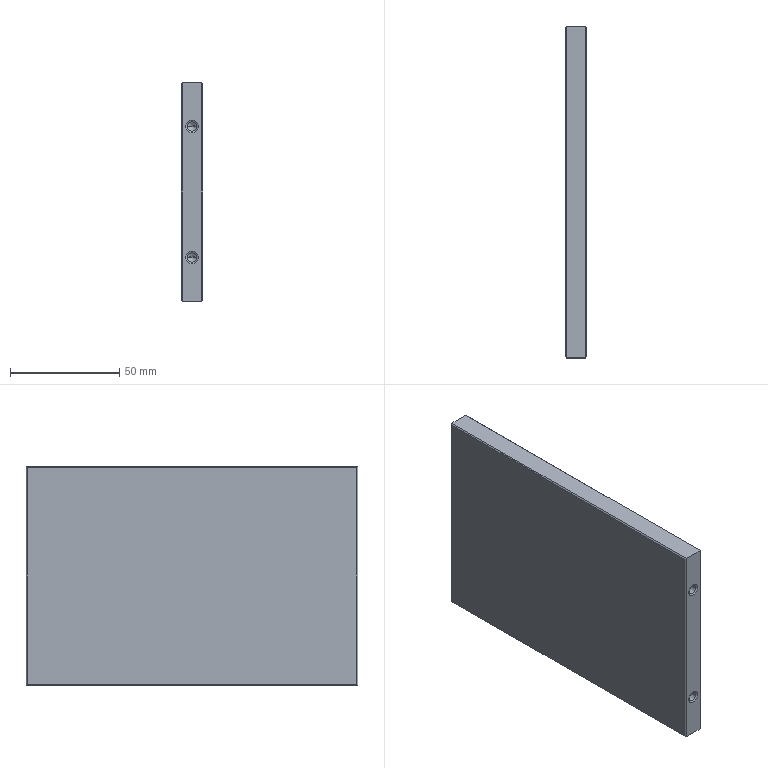Part | NX | 1 solid | 38 faces | box 10 x 151.9 x 100 mm | volume 150921 mm3 | cone 16 | plane 14 | cylinder 8 | commonest cylinder face diameters 4.2 x8
STEP:
#1=CARTESIAN_POINT('',(-4.5,-74.75,0.));
#2=VERTEX_POINT('',#1);
#3=CARTESIAN_POINT('',(4.5,-74.75,0.));
#4=VERTEX_POINT('',#3);
#5=CARTESIAN_POINT('',(0.,-74.75,0.));
#6=DIRECTION('',(1.,0.,0.));
#7=VECTOR('',#6,1000.);
#8=LINE('',#5,#7);
#9=EDGE_CURVE('',#2,#4,#8,.T.);
#10=ORIENTED_EDGE('',*,*,#9,.F.);
#11=CARTESIAN_POINT('',(-4.5,77.15,0.));
#12=VERTEX_POINT('',#11);
#13=CARTESIAN_POINT('',(-4.5,0.,0.));
#14=DIRECTION('',(0.,-1.,0.));
#15=VECTOR('',#14,1000.);
#16=LINE('',#13,#15);
#17=EDGE_CURVE('',#12,#2,#16,.T.);
#18=ORIENTED_EDGE('',*,*,#17,.F.);
#19=CARTESIAN_POINT('',(4.5,77.15,0.));
#20=VERTEX_POINT('',#19);
#21=CARTESIAN_POINT('',(0.,77.15,0.));
#22=DIRECTION('',(-1.,0.,0.));
#23=VECTOR('',#22,1000.);
#24=LINE('',#21,#23);
#25=EDGE_CURVE('',#20,#12,#24,.T.);
#26=ORIENTED_EDGE('',*,*,#25,.F.);
#27=CARTESIAN_POINT('',(4.5,0.,0.));
#28=DIRECTION('',(0.,1.,0.));
#29=VECTOR('',#28,1000.);
#30=LINE('',#27,#29);
#31=EDGE_CURVE('',#4,#20,#30,.T.);
#32=ORIENTED_EDGE('',*,*,#31,.F.);
#33=EDGE_LOOP('',(#10,#18,#26,#32));
#34=FACE_BOUND('',#33,.T.);
#35=CARTESIAN_POINT('',(0.,0.,0.));
#36=DIRECTION('',(0.,0.,1.));
#37=DIRECTION('',(1.,0.,0.));
#38=AXIS2_PLACEMENT_3D('',#35,#36,#37);
#39=PLANE('',#38);
#40=ADVANCED_FACE('',(#34),#39,.F.);
#41=CARTESIAN_POINT('',(-5.,-74.25,0.5));
#42=VERTEX_POINT('',#41);
#43=CARTESIAN_POINT('',(-4.5,-74.75,0.));
#44=DIRECTION('',(0.5774,-0.5774,-0.5774));
#45=VECTOR('',#44,1000.);
#46=LINE('',#43,#45);
#47=EDGE_CURVE('',#42,#2,#46,.T.);
#48=ORIENTED_EDGE('',*,*,#47,.F.);
#49=CARTESIAN_POINT('',(-5.,76.65,0.5));
#50=VERTEX_POINT('',#49);
#51=CARTESIAN_POINT('',(-5.,0.,0.5));
#52=DIRECTION('',(0.,-1.,0.));
#53=VECTOR('',#52,1000.);
#54=LINE('',#51,#53);
#55=EDGE_CURVE('',#50,#42,#54,.T.);
#56=ORIENTED_EDGE('',*,*,#55,.F.);
#57=CARTESIAN_POINT('',(-4.5,77.15,0.));
#58=DIRECTION('',(-0.5774,-0.5774,0.5774));
#59=VECTOR('',#58,1000.);
#60=LINE('',#57,#59);
#61=EDGE_CURVE('',#12,#50,#60,.T.);
#62=ORIENTED_EDGE('',*,*,#61,.F.);
#63=ORIENTED_EDGE('',*,*,#17,.T.);
#64=EDGE_LOOP('',(#48,#56,#62,#63));
#65=FACE_BOUND('',#64,.T.);
#66=CARTESIAN_POINT('',(-4.5,76.65,0.));
#67=DIRECTION('',(-0.7071,0.,-0.7071));
#68=DIRECTION('',(-0.7071,0.,0.7071));
#69=AXIS2_PLACEMENT_3D('',#66,#67,#68);
#70=PLANE('',#69);
#71=ADVANCED_FACE('',(#65),#70,.T.);
#72=CARTESIAN_POINT('',(5.,76.65,0.5));
#73=VERTEX_POINT('',#72);
#74=CARTESIAN_POINT('',(5.,-74.25,0.5));
#75=VERTEX_POINT('',#74);
#76=CARTESIAN_POINT('',(5.,0.,0.5));
#77=DIRECTION('',(0.,-1.,0.));
#78=VECTOR('',#77,1000.);
#79=LINE('',#76,#78);
#80=EDGE_CURVE('',#73,#75,#79,.T.);
#81=ORIENTED_EDGE('',*,*,#80,.F.);
#82=CARTESIAN_POINT('',(5.,76.65,99.5));
#83=VERTEX_POINT('',#82);
#84=CARTESIAN_POINT('',(5.,76.65,0.));
#85=DIRECTION('',(0.,0.,-1.));
#86=VECTOR('',#85,1000.);
#87=LINE('',#84,#86);
#88=EDGE_CURVE('',#83,#73,#87,.T.);
#89=ORIENTED_EDGE('',*,*,#88,.F.);
#90=CARTESIAN_POINT('',(5.,-74.25,99.5));
#91=VERTEX_POINT('',#90);
#92=CARTESIAN_POINT('',(5.,0.,99.5));
#93=DIRECTION('',(0.,-1.,0.));
#94=VECTOR('',#93,1000.);
#95=LINE('',#92,#94);
#96=EDGE_CURVE('',#83,#91,#95,.T.);
#97=ORIENTED_EDGE('',*,*,#96,.T.);
#98=CARTESIAN_POINT('',(5.,-74.25,0.));
#99=DIRECTION('',(0.,0.,1.));
#100=VECTOR('',#99,1000.);
#101=LINE('',#98,#100);
#102=EDGE_CURVE('',#75,#91,#101,.T.);
#103=ORIENTED_EDGE('',*,*,#102,.F.);
#104=EDGE_LOOP('',(#81,#89,#97,#103));
#105=FACE_BOUND('',#104,.T.);
#106=CARTESIAN_POINT('',(5.,-77.15,0.));
#107=DIRECTION('',(1.,0.,0.));
#108=DIRECTION('',(0.,1.,0.));
#109=AXIS2_PLACEMENT_3D('',#106,#107,#108);
#110=PLANE('',#109);
#111=ADVANCED_FACE('',(#105),#110,.T.);
#112=ORIENTED_EDGE('',*,*,#31,.T.);
#113=CARTESIAN_POINT('',(4.5,77.15,0.));
#114=DIRECTION('',(-0.5774,0.5774,-0.5774));
#115=VECTOR('',#114,1000.);
#116=LINE('',#113,#115);
#117=EDGE_CURVE('',#73,#20,#116,.T.);
#118=ORIENTED_EDGE('',*,*,#117,.F.);
#119=ORIENTED_EDGE('',*,*,#80,.T.);
#120=CARTESIAN_POINT('',(4.5,-74.75,0.));
#121=DIRECTION('',(-0.5774,-0.5774,-0.5774));
#122=VECTOR('',#121,1000.);
#123=LINE('',#120,#122);
#124=EDGE_CURVE('',#75,#4,#123,.T.);
#125=ORIENTED_EDGE('',*,*,#124,.T.);
#126=EDGE_LOOP('',(#112,#118,#119,#125));
#127=FACE_BOUND('',#126,.T.);
#128=CARTESIAN_POINT('',(4.5,-77.15,0.));
#129=DIRECTION('',(0.7071,0.,-0.7071));
#130=DIRECTION('',(0.,-1.,0.));
#131=AXIS2_PLACEMENT_3D('',#128,#129,#130);
#132=PLANE('',#131);
#133=ADVANCED_FACE('',(#127),#132,.T.);
#134=CARTESIAN_POINT('',(4.5,-74.75,100.));
#135=VERTEX_POINT('',#134);
#136=CARTESIAN_POINT('',(104.5,25.25,0.));
#137=DIRECTION('',(0.5774,0.5774,-0.5774));
#138=VECTOR('',#137,1000.);
#139=LINE('',#136,#138);
#140=EDGE_CURVE('',#135,#91,#139,.T.);
#141=ORIENTED_EDGE('',*,*,#140,.T.);
#142=ORIENTED_EDGE('',*,*,#96,.F.);
#143=CARTESIAN_POINT('',(4.5,77.15,100.));
#144=VERTEX_POINT('',#143);
#145=CARTESIAN_POINT('',(104.5,-22.85,0.));
#146=DIRECTION('',(-0.5774,0.5774,0.5774));
#147=VECTOR('',#146,1000.);
#148=LINE('',#145,#147);
#149=EDGE_CURVE('',#83,#144,#148,.T.);
#150=ORIENTED_EDGE('',*,*,#149,.T.);
#151=CARTESIAN_POINT('',(4.5,0.,100.));
#152=DIRECTION('',(0.,1.,0.));
#153=VECTOR('',#152,1000.);
#154=LINE('',#151,#153);
#155=EDGE_CURVE('',#135,#144,#154,.T.);
#156=ORIENTED_EDGE('',*,*,#155,.F.);
#157=EDGE_LOOP('',(#141,#142,#150,#156));
#158=FACE_BOUND('',#157,.T.);
#159=CARTESIAN_POINT('',(4.5,-77.15,100.));
#160=DIRECTION('',(-0.7071,0.,-0.7071));
#161=DIRECTION('',(-0.7071,0.,0.7071));
#162=AXIS2_PLACEMENT_3D('',#159,#160,#161);
#163=PLANE('',#162);
#164=ADVANCED_FACE('',(#158),#163,.F.);
#165=CARTESIAN_POINT('',(-4.5,-74.75,100.));
#166=VERTEX_POINT('',#165);
#167=CARTESIAN_POINT('',(-4.5,-74.75,0.));
#168=DIRECTION('',(0.,0.,1.));
#169=VECTOR('',#168,1000.);
#170=LINE('',#167,#169);
#171=EDGE_CURVE('',#2,#166,#170,.T.);
#172=ORIENTED_EDGE('',*,*,#171,.T.);
#173=CARTESIAN_POINT('',(-5.,-74.25,99.5));
#174=VERTEX_POINT('',#173);
#175=CARTESIAN_POINT('',(-104.5,25.25,0.));
#176=DIRECTION('',(0.5774,-0.5774,0.5774));
#177=VECTOR('',#176,1000.);
#178=LINE('',#175,#177);
#179=EDGE_CURVE('',#174,#166,#178,.T.);
#180=ORIENTED_EDGE('',*,*,#179,.F.);
#181=CARTESIAN_POINT('',(-5.,-74.25,0.));
#182=DIRECTION('',(0.,0.,-1.));
#183=VECTOR('',#182,1000.);
#184=LINE('',#181,#183);
#185=EDGE_CURVE('',#174,#42,#184,.T.);
#186=ORIENTED_EDGE('',*,*,#185,.T.);
#187=ORIENTED_EDGE('',*,*,#47,.T.);
#188=EDGE_LOOP('',(#172,#180,#186,#187));
#189=FACE_BOUND('',#188,.T.);
#190=CARTESIAN_POINT('',(-4.5,-74.75,0.));
#191=DIRECTION('',(-0.7071,-0.7071,0.));
#192=DIRECTION('',(-0.7071,0.7071,0.));
#193=AXIS2_PLACEMENT_3D('',#190,#191,#192);
#194=PLANE('',#193);
#195=ADVANCED_FACE('',(#189),#194,.T.);
#196=ORIENTED_EDGE('',*,*,#25,.T.);
#197=CARTESIAN_POINT('',(-4.5,77.15,100.));
#198=VERTEX_POINT('',#197);
#199=CARTESIAN_POINT('',(-4.5,77.15,0.));
#200=DIRECTION('',(0.,0.,-1.));
#201=VECTOR('',#200,1000.);
#202=LINE('',#199,#201);
#203=EDGE_CURVE('',#198,#12,#202,.T.);
#204=ORIENTED_EDGE('',*,*,#203,.F.);
#205=CARTESIAN_POINT('',(0.,77.15,100.));
#206=DIRECTION('',(-1.,0.,0.));
#207=VECTOR('',#206,1000.);
#208=LINE('',#205,#207);
#209=EDGE_CURVE('',#144,#198,#208,.T.);
#210=ORIENTED_EDGE('',*,*,#209,.F.);
#211=CARTESIAN_POINT('',(4.5,77.15,0.));
#212=DIRECTION('',(0.,0.,1.));
#213=VECTOR('',#212,1000.);
#214=LINE('',#211,#213);
#215=EDGE_CURVE('',#20,#144,#214,.T.);
#216=ORIENTED_EDGE('',*,*,#215,.F.);
#217=EDGE_LOOP('',(#196,#204,#210,#216));
#218=FACE_BOUND('',#217,.T.);
#219=CARTESIAN_POINT('',(2.86,77.15,20.));
#220=VERTEX_POINT('',#219);
#221=CARTESIAN_POINT('',(-2.86,77.15,20.));
#222=VERTEX_POINT('',#221);
#223=CARTESIAN_POINT('',(0.,77.15,20.));
#224=DIRECTION('',(0.,1.,0.));
#225=DIRECTION('',(1.,0.,0.));
#226=AXIS2_PLACEMENT_3D('',#223,#224,#225);
#227=CIRCLE('',#226,2.86);
#228=EDGE_CURVE('',#220,#222,#227,.T.);
#229=ORIENTED_EDGE('',*,*,#228,.F.);
#230=CARTESIAN_POINT('',(0.,77.15,20.));
#231=DIRECTION('',(0.,1.,0.));
#232=DIRECTION('',(1.,0.,0.));
#233=AXIS2_PLACEMENT_3D('',#230,#231,#232);
#234=CIRCLE('',#233,2.86);
#235=EDGE_CURVE('',#222,#220,#234,.T.);
#236=ORIENTED_EDGE('',*,*,#235,.F.);
#237=EDGE_LOOP('',(#229,#236));
#238=FACE_BOUND('',#237,.T.);
#239=CARTESIAN_POINT('',(-2.86,77.15,80.));
#240=VERTEX_POINT('',#239);
#241=CARTESIAN_POINT('',(2.86,77.15,80.));
#242=VERTEX_POINT('',#241);
#243=CARTESIAN_POINT('',(0.,77.15,80.));
#244=DIRECTION('',(0.,1.,0.));
#245=DIRECTION('',(1.,0.,0.));
#246=AXIS2_PLACEMENT_3D('',#243,#244,#245);
#247=CIRCLE('',#246,2.86);
#248=EDGE_CURVE('',#240,#242,#247,.T.);
#249=ORIENTED_EDGE('',*,*,#248,.F.);
#250=CARTESIAN_POINT('',(0.,77.15,80.));
#251=DIRECTION('',(0.,1.,0.));
#252=DIRECTION('',(1.,0.,0.));
#253=AXIS2_PLACEMENT_3D('',#250,#251,#252);
#254=CIRCLE('',#253,2.86);
#255=EDGE_CURVE('',#242,#240,#254,.T.);
#256=ORIENTED_EDGE('',*,*,#255,.F.);
#257=EDGE_LOOP('',(#249,#256));
#258=FACE_BOUND('',#257,.T.);
#259=CARTESIAN_POINT('',(5.,77.15,0.));
#260=DIRECTION('',(0.,1.,0.));
#261=DIRECTION('',(1.,0.,0.));
#262=AXIS2_PLACEMENT_3D('',#259,#260,#261);
#263=PLANE('',#262);
#264=ADVANCED_FACE('',(#218,#238,#258),#263,.T.);
#265=ORIENTED_EDGE('',*,*,#124,.F.);
#266=ORIENTED_EDGE('',*,*,#102,.T.);
#267=ORIENTED_EDGE('',*,*,#140,.F.);
#268=CARTESIAN_POINT('',(4.5,-74.75,0.));
#269=DIRECTION('',(0.,0.,-1.));
#270=VECTOR('',#269,1000.);
#271=LINE('',#268,#270);
#272=EDGE_CURVE('',#135,#4,#271,.T.);
#273=ORIENTED_EDGE('',*,*,#272,.T.);
#274=EDGE_LOOP('',(#265,#266,#267,#273));
#275=FACE_BOUND('',#274,.T.);
#276=CARTESIAN_POINT('',(5.,-74.25,0.5));
#277=DIRECTION('',(0.7071,-0.7071,0.));
#278=DIRECTION('',(0.,0.,-1.));
#279=AXIS2_PLACEMENT_3D('',#276,#277,#278);
#280=PLANE('',#279);
#281=ADVANCED_FACE('',(#275),#280,.T.);
#282=CARTESIAN_POINT('',(0.,-74.75,100.));
#283=DIRECTION('',(1.,0.,0.));
#284=VECTOR('',#283,1000.);
#285=LINE('',#282,#284);
#286=EDGE_CURVE('',#166,#135,#285,.T.);
#287=ORIENTED_EDGE('',*,*,#286,.T.);
#288=ORIENTED_EDGE('',*,*,#155,.T.);
#289=ORIENTED_EDGE('',*,*,#209,.T.);
#290=CARTESIAN_POINT('',(-4.5,0.,100.));
#291=DIRECTION('',(0.,-1.,0.));
#292=VECTOR('',#291,1000.);
#293=LINE('',#290,#292);
#294=EDGE_CURVE('',#198,#166,#293,.T.);
#295=ORIENTED_EDGE('',*,*,#294,.T.);
#296=EDGE_LOOP('',(#287,#288,#289,#295));
#297=FACE_BOUND('',#296,.T.);
#298=CARTESIAN_POINT('',(0.,0.,100.));
#299=DIRECTION('',(0.,0.,1.));
#300=DIRECTION('',(1.,0.,0.));
#301=AXIS2_PLACEMENT_3D('',#298,#299,#300);
#302=PLANE('',#301);
#303=ADVANCED_FACE('',(#297),#302,.T.);
#304=ORIENTED_EDGE('',*,*,#294,.F.);
#305=CARTESIAN_POINT('',(-5.,76.65,99.5));
#306=VERTEX_POINT('',#305);
#307=CARTESIAN_POINT('',(-104.5,-22.85,0.));
#308=DIRECTION('',(-0.5774,-0.5774,-0.5774));
#309=VECTOR('',#308,1000.);
#310=LINE('',#307,#309);
#311=EDGE_CURVE('',#198,#306,#310,.T.);
#312=ORIENTED_EDGE('',*,*,#311,.T.);
#313=CARTESIAN_POINT('',(-5.,0.,99.5));
#314=DIRECTION('',(0.,1.,0.));
#315=VECTOR('',#314,1000.);
#316=LINE('',#313,#315);
#317=EDGE_CURVE('',#174,#306,#316,.T.);
#318=ORIENTED_EDGE('',*,*,#317,.F.);
#319=ORIENTED_EDGE('',*,*,#179,.T.);
#320=EDGE_LOOP('',(#304,#312,#318,#319));
#321=FACE_BOUND('',#320,.T.);
#322=CARTESIAN_POINT('',(-4.5,76.65,100.));
#323=DIRECTION('',(0.7071,0.,-0.7071));
#324=DIRECTION('',(0.,-1.,0.));
#325=AXIS2_PLACEMENT_3D('',#322,#323,#324);
#326=PLANE('',#325);
#327=ADVANCED_FACE('',(#321),#326,.F.);
#328=ORIENTED_EDGE('',*,*,#55,.T.);
#329=ORIENTED_EDGE('',*,*,#185,.F.);
#330=ORIENTED_EDGE('',*,*,#317,.T.);
#331=CARTESIAN_POINT('',(-5.,76.65,0.));
#332=DIRECTION('',(0.,0.,1.));
#333=VECTOR('',#332,1000.);
#334=LINE('',#331,#333);
#335=EDGE_CURVE('',#50,#306,#334,.T.);
#336=ORIENTED_EDGE('',*,*,#335,.F.);
#337=EDGE_LOOP('',(#328,#329,#330,#336));
#338=FACE_BOUND('',#337,.T.);
#339=CARTESIAN_POINT('',(-5.,77.15,0.));
#340=DIRECTION('',(-1.,0.,0.));
#341=DIRECTION('',(0.,0.,1.));
#342=AXIS2_PLACEMENT_3D('',#339,#340,#341);
#343=PLANE('',#342);
#344=ADVANCED_FACE('',(#338),#343,.T.);
#345=ORIENTED_EDGE('',*,*,#61,.T.);
#346=ORIENTED_EDGE('',*,*,#335,.T.);
#347=ORIENTED_EDGE('',*,*,#311,.F.);
#348=ORIENTED_EDGE('',*,*,#203,.T.);
#349=EDGE_LOOP('',(#345,#346,#347,#348));
#350=FACE_BOUND('',#349,.T.);
#351=CARTESIAN_POINT('',(-5.,76.65,0.));
#352=DIRECTION('',(-0.7071,0.7071,0.));
#353=DIRECTION('',(0.,0.,1.));
#354=AXIS2_PLACEMENT_3D('',#351,#352,#353);
#355=PLANE('',#354);
#356=ADVANCED_FACE('',(#350),#355,.T.);
#357=ORIENTED_EDGE('',*,*,#9,.T.);
#358=ORIENTED_EDGE('',*,*,#272,.F.);
#359=ORIENTED_EDGE('',*,*,#286,.F.);
#360=ORIENTED_EDGE('',*,*,#171,.F.);
#361=EDGE_LOOP('',(#357,#358,#359,#360));
#362=FACE_BOUND('',#361,.T.);
#363=CARTESIAN_POINT('',(-2.86,-74.75,20.));
#364=VERTEX_POINT('',#363);
#365=CARTESIAN_POINT('',(2.86,-74.75,20.));
#366=VERTEX_POINT('',#365);
#367=CARTESIAN_POINT('',(0.,-74.75,20.));
#368=DIRECTION('',(0.,-1.,0.));
#369=DIRECTION('',(-1.,0.,0.));
#370=AXIS2_PLACEMENT_3D('',#367,#368,#369);
#371=CIRCLE('',#370,2.86);
#372=EDGE_CURVE('',#364,#366,#371,.T.);
#373=ORIENTED_EDGE('',*,*,#372,.F.);
#374=CARTESIAN_POINT('',(0.,-74.75,20.));
#375=DIRECTION('',(0.,-1.,0.));
#376=DIRECTION('',(-1.,0.,0.));
#377=AXIS2_PLACEMENT_3D('',#374,#375,#376);
#378=CIRCLE('',#377,2.86);
#379=EDGE_CURVE('',#366,#364,#378,.T.);
#380=ORIENTED_EDGE('',*,*,#379,.F.);
#381=EDGE_LOOP('',(#373,#380));
#382=FACE_BOUND('',#381,.T.);
#383=CARTESIAN_POINT('',(-2.86,-74.75,80.));
#384=VERTEX_POINT('',#383);
#385=CARTESIAN_POINT('',(2.86,-74.75,80.));
#386=VERTEX_POINT('',#385);
#387=CARTESIAN_POINT('',(0.,-74.75,80.));
#388=DIRECTION('',(0.,-1.,0.));
#389=DIRECTION('',(-1.,0.,0.));
#390=AXIS2_PLACEMENT_3D('',#387,#388,#389);
#391=CIRCLE('',#390,2.86);
#392=EDGE_CURVE('',#384,#386,#391,.T.);
#393=ORIENTED_EDGE('',*,*,#392,.F.);
#394=CARTESIAN_POINT('',(0.,-74.75,80.));
#395=DIRECTION('',(0.,-1.,0.));
#396=DIRECTION('',(-1.,0.,0.));
#397=AXIS2_PLACEMENT_3D('',#394,#395,#396);
#398=CIRCLE('',#397,2.86);
#399=EDGE_CURVE('',#386,#384,#398,.T.);
#400=ORIENTED_EDGE('',*,*,#399,.F.);
#401=EDGE_LOOP('',(#393,#400));
#402=FACE_BOUND('',#401,.T.);
#403=CARTESIAN_POINT('',(-5.,-74.75,0.));
#404=DIRECTION('',(0.,-1.,0.));
#405=DIRECTION('',(0.,0.,-1.));
#406=AXIS2_PLACEMENT_3D('',#403,#404,#405);
#407=PLANE('',#406);
#408=ADVANCED_FACE('',(#362,#382,#402),#407,.T.);
#409=ORIENTED_EDGE('',*,*,#215,.T.);
#410=ORIENTED_EDGE('',*,*,#149,.F.);
#411=ORIENTED_EDGE('',*,*,#88,.T.);
#412=ORIENTED_EDGE('',*,*,#117,.T.);
#413=EDGE_LOOP('',(#409,#410,#411,#412));
#414=FACE_BOUND('',#413,.T.);
#415=CARTESIAN_POINT('',(4.5,77.15,0.));
#416=DIRECTION('',(0.7071,0.7071,0.));
#417=DIRECTION('',(0.,0.,-1.));
#418=AXIS2_PLACEMENT_3D('',#415,#416,#417);
#419=PLANE('',#418);
#420=ADVANCED_FACE('',(#414),#419,.T.);
#421=CARTESIAN_POINT('',(2.1,-74.311,20.));
#422=VERTEX_POINT('',#421);
#423=CARTESIAN_POINT('',(-2.1,-74.311,20.));
#424=VERTEX_POINT('',#423);
#425=CARTESIAN_POINT('',(0.,-74.311,20.));
#426=DIRECTION('',(0.,-1.,0.));
#427=DIRECTION('',(-1.,0.,0.));
#428=AXIS2_PLACEMENT_3D('',#425,#426,#427);
#429=CIRCLE('',#428,2.1);
#430=EDGE_CURVE('',#422,#424,#429,.T.);
#431=ORIENTED_EDGE('',*,*,#430,.T.);
#432=CARTESIAN_POINT('',(-2.1,-59.95,20.));
#433=VERTEX_POINT('',#432);
#434=CARTESIAN_POINT('',(-2.1,-74.75,20.));
#435=DIRECTION('',(0.,-1.,0.));
#436=VECTOR('',#435,1000.);
#437=LINE('',#434,#436);
#438=EDGE_CURVE('',#424,#433,#437,.F.);
#439=ORIENTED_EDGE('',*,*,#438,.T.);
#440=CARTESIAN_POINT('',(2.1,-59.95,20.));
#441=VERTEX_POINT('',#440);
#442=CARTESIAN_POINT('',(0.,-59.95,20.));
#443=DIRECTION('',(0.,-1.,0.));
#444=DIRECTION('',(-1.,0.,0.));
#445=AXIS2_PLACEMENT_3D('',#442,#443,#444);
#446=CIRCLE('',#445,2.1);
#447=EDGE_CURVE('',#441,#433,#446,.T.);
#448=ORIENTED_EDGE('',*,*,#447,.F.);
#449=CARTESIAN_POINT('',(2.1,-74.75,20.));
#450=DIRECTION('',(0.,-1.,0.));
#451=VECTOR('',#450,1000.);
#452=LINE('',#449,#451);
#453=EDGE_CURVE('',#422,#441,#452,.F.);
#454=ORIENTED_EDGE('',*,*,#453,.F.);
#455=EDGE_LOOP('',(#431,#439,#448,#454));
#456=FACE_BOUND('',#455,.T.);
#457=CARTESIAN_POINT('',(0.,-74.75,20.));
#458=DIRECTION('',(0.,-1.,0.));
#459=DIRECTION('',(-1.,0.,0.));
#460=AXIS2_PLACEMENT_3D('',#457,#458,#459);
#461=CYLINDRICAL_SURFACE('',#460,2.1);
#462=ADVANCED_FACE('',(#456),#461,.F.);
#463=ORIENTED_EDGE('',*,*,#430,.F.);
#464=CARTESIAN_POINT('',(2.1,-74.311,20.));
#465=DIRECTION('',(0.866,-0.5,0.));
#466=VECTOR('',#465,1000.);
#467=LINE('',#464,#466);
#468=EDGE_CURVE('',#422,#366,#467,.T.);
#469=ORIENTED_EDGE('',*,*,#468,.T.);
#470=ORIENTED_EDGE('',*,*,#379,.T.);
#471=CARTESIAN_POINT('',(-2.1,-74.311,20.));
#472=DIRECTION('',(-0.866,-0.5,0.));
#473=VECTOR('',#472,1000.);
#474=LINE('',#471,#473);
#475=EDGE_CURVE('',#424,#364,#474,.T.);
#476=ORIENTED_EDGE('',*,*,#475,.F.);
#477=EDGE_LOOP('',(#463,#469,#470,#476));
#478=FACE_BOUND('',#477,.T.);
#479=CARTESIAN_POINT('',(0.,-74.311,20.));
#480=DIRECTION('',(0.,-1.,0.));
#481=DIRECTION('',(-1.,0.,0.));
#482=AXIS2_PLACEMENT_3D('',#479,#480,#481);
#483=CONICAL_SURFACE('',#482,2.1,1.047);
#484=ADVANCED_FACE('',(#478),#483,.F.);
#485=CARTESIAN_POINT('',(2.1,76.711,80.));
#486=VERTEX_POINT('',#485);
#487=CARTESIAN_POINT('',(-2.1,76.711,80.));
#488=VERTEX_POINT('',#487);
#489=CARTESIAN_POINT('',(0.,76.711,80.));
#490=DIRECTION('',(0.,1.,0.));
#491=DIRECTION('',(1.,0.,0.));
#492=AXIS2_PLACEMENT_3D('',#489,#490,#491);
#493=CIRCLE('',#492,2.1);
#494=EDGE_CURVE('',#486,#488,#493,.T.);
#495=ORIENTED_EDGE('',*,*,#494,.T.);
#496=CARTESIAN_POINT('',(-2.1,62.35,80.));
#497=VERTEX_POINT('',#496);
#498=CARTESIAN_POINT('',(-2.1,77.15,80.));
#499=DIRECTION('',(0.,1.,0.));
#500=VECTOR('',#499,1000.);
#501=LINE('',#498,#500);
#502=EDGE_CURVE('',#488,#497,#501,.F.);
#503=ORIENTED_EDGE('',*,*,#502,.T.);
#504=CARTESIAN_POINT('',(2.1,62.35,80.));
#505=VERTEX_POINT('',#504);
#506=CARTESIAN_POINT('',(0.,62.35,80.));
#507=DIRECTION('',(0.,1.,0.));
#508=DIRECTION('',(1.,0.,0.));
#509=AXIS2_PLACEMENT_3D('',#506,#507,#508);
#510=CIRCLE('',#509,2.1);
#511=EDGE_CURVE('',#505,#497,#510,.T.);
#512=ORIENTED_EDGE('',*,*,#511,.F.);
#513=CARTESIAN_POINT('',(2.1,77.15,80.));
#514=DIRECTION('',(0.,1.,0.));
#515=VECTOR('',#514,1000.);
#516=LINE('',#513,#515);
#517=EDGE_CURVE('',#486,#505,#516,.F.);
#518=ORIENTED_EDGE('',*,*,#517,.F.);
#519=EDGE_LOOP('',(#495,#503,#512,#518));
#520=FACE_BOUND('',#519,.T.);
#521=CARTESIAN_POINT('',(0.,77.15,80.));
#522=DIRECTION('',(0.,1.,0.));
#523=DIRECTION('',(1.,0.,0.));
#524=AXIS2_PLACEMENT_3D('',#521,#522,#523);
#525=CYLINDRICAL_SURFACE('',#524,2.1);
#526=ADVANCED_FACE('',(#520),#525,.F.);
#527=ORIENTED_EDGE('',*,*,#447,.T.);
#528=CARTESIAN_POINT('',(0.,-58.688,20.));
#529=VERTEX_POINT('',#528);
#530=CARTESIAN_POINT('',(-2.1,-59.95,20.));
#531=DIRECTION('',(-0.8572,-0.515,0.));
#532=VECTOR('',#531,1000.);
#533=LINE('',#530,#532);
#534=EDGE_CURVE('',#529,#433,#533,.T.);
#535=ORIENTED_EDGE('',*,*,#534,.F.);
#536=CARTESIAN_POINT('',(2.1,-59.95,20.));
#537=DIRECTION('',(0.8572,-0.515,0.));
#538=VECTOR('',#537,1000.);
#539=LINE('',#536,#538);
#540=EDGE_CURVE('',#529,#441,#539,.T.);
#541=ORIENTED_EDGE('',*,*,#540,.T.);
#542=EDGE_LOOP('',(#527,#535,#541));
#543=FACE_BOUND('',#542,.T.);
#544=CARTESIAN_POINT('',(0.,-59.95,20.));
#545=DIRECTION('',(0.,-1.,0.));
#546=DIRECTION('',(-1.,0.,0.));
#547=AXIS2_PLACEMENT_3D('',#544,#545,#546);
#548=CONICAL_SURFACE('',#547,2.1,1.03);
#549=ADVANCED_FACE('',(#543),#548,.F.);
#550=CARTESIAN_POINT('',(-2.1,-59.95,80.));
#551=VERTEX_POINT('',#550);
#552=CARTESIAN_POINT('',(2.1,-59.95,80.));
#553=VERTEX_POINT('',#552);
#554=CARTESIAN_POINT('',(0.,-59.95,80.));
#555=DIRECTION('',(0.,-1.,0.));
#556=DIRECTION('',(-1.,0.,0.));
#557=AXIS2_PLACEMENT_3D('',#554,#555,#556);
#558=CIRCLE('',#557,2.1);
#559=EDGE_CURVE('',#551,#553,#558,.T.);
#560=ORIENTED_EDGE('',*,*,#559,.F.);
#561=CARTESIAN_POINT('',(-2.1,-74.311,80.));
#562=VERTEX_POINT('',#561);
#563=CARTESIAN_POINT('',(-2.1,-74.75,80.));
#564=DIRECTION('',(0.,-1.,0.));
#565=VECTOR('',#564,1000.);
#566=LINE('',#563,#565);
#567=EDGE_CURVE('',#562,#551,#566,.F.);
#568=ORIENTED_EDGE('',*,*,#567,.F.);
#569=CARTESIAN_POINT('',(2.1,-74.311,80.));
#570=VERTEX_POINT('',#569);
#571=CARTESIAN_POINT('',(0.,-74.311,80.));
#572=DIRECTION('',(0.,-1.,0.));
#573=DIRECTION('',(-1.,0.,0.));
#574=AXIS2_PLACEMENT_3D('',#571,#572,#573);
#575=CIRCLE('',#574,2.1);
#576=EDGE_CURVE('',#562,#570,#575,.T.);
#577=ORIENTED_EDGE('',*,*,#576,.T.);
#578=CARTESIAN_POINT('',(2.1,-74.75,80.));
#579=DIRECTION('',(0.,-1.,0.));
#580=VECTOR('',#579,1000.);
#581=LINE('',#578,#580);
#582=EDGE_CURVE('',#570,#553,#581,.F.);
#583=ORIENTED_EDGE('',*,*,#582,.T.);
#584=EDGE_LOOP('',(#560,#568,#577,#583));
#585=FACE_BOUND('',#584,.T.);
#586=CARTESIAN_POINT('',(0.,-74.75,80.));
#587=DIRECTION('',(0.,-1.,0.));
#588=DIRECTION('',(-1.,0.,0.));
#589=AXIS2_PLACEMENT_3D('',#586,#587,#588);
#590=CYLINDRICAL_SURFACE('',#589,2.1);
#591=ADVANCED_FACE('',(#585),#590,.F.);
#592=ORIENTED_EDGE('',*,*,#494,.F.);
#593=CARTESIAN_POINT('',(2.1,76.711,80.));
#594=DIRECTION('',(0.866,0.5,0.));
#595=VECTOR('',#594,1000.);
#596=LINE('',#593,#595);
#597=EDGE_CURVE('',#486,#242,#596,.T.);
#598=ORIENTED_EDGE('',*,*,#597,.T.);
#599=ORIENTED_EDGE('',*,*,#255,.T.);
#600=CARTESIAN_POINT('',(-2.1,76.711,80.));
#601=DIRECTION('',(-0.866,0.5,0.));
#602=VECTOR('',#601,1000.);
#603=LINE('',#600,#602);
#604=EDGE_CURVE('',#488,#240,#603,.T.);
#605=ORIENTED_EDGE('',*,*,#604,.F.);
#606=EDGE_LOOP('',(#592,#598,#599,#605));
#607=FACE_BOUND('',#606,.T.);
#608=CARTESIAN_POINT('',(0.,76.711,80.));
#609=DIRECTION('',(0.,1.,0.));
#610=DIRECTION('',(1.,0.,0.));
#611=AXIS2_PLACEMENT_3D('',#608,#609,#610);
#612=CONICAL_SURFACE('',#611,2.1,1.047);
#613=ADVANCED_FACE('',(#607),#612,.F.);
#614=CARTESIAN_POINT('',(0.,-58.688,80.));
#615=VERTEX_POINT('',#614);
#616=CARTESIAN_POINT('',(2.1,-59.95,80.));
#617=DIRECTION('',(0.8572,-0.515,0.));
#618=VECTOR('',#617,1000.);
#619=LINE('',#616,#618);
#620=EDGE_CURVE('',#615,#553,#619,.T.);
#621=ORIENTED_EDGE('',*,*,#620,.T.);
#622=CARTESIAN_POINT('',(0.,-59.95,80.));
#623=DIRECTION('',(0.,-1.,0.));
#624=DIRECTION('',(-1.,0.,0.));
#625=AXIS2_PLACEMENT_3D('',#622,#623,#624);
#626=CIRCLE('',#625,2.1);
#627=EDGE_CURVE('',#553,#551,#626,.T.);
#628=ORIENTED_EDGE('',*,*,#627,.T.);
#629=CARTESIAN_POINT('',(-2.1,-59.95,80.));
#630=DIRECTION('',(-0.8572,-0.515,0.));
#631=VECTOR('',#630,1000.);
#632=LINE('',#629,#631);
#633=EDGE_CURVE('',#615,#551,#632,.T.);
#634=ORIENTED_EDGE('',*,*,#633,.F.);
#635=EDGE_LOOP('',(#621,#628,#634));
#636=FACE_BOUND('',#635,.T.);
#637=CARTESIAN_POINT('',(0.,-59.95,80.));
#638=DIRECTION('',(0.,-1.,0.));
#639=DIRECTION('',(-1.,0.,0.));
#640=AXIS2_PLACEMENT_3D('',#637,#638,#639);
#641=CONICAL_SURFACE('',#640,2.1,1.03);
#642=ADVANCED_FACE('',(#636),#641,.F.);
#643=ORIENTED_EDGE('',*,*,#576,.F.);
#644=CARTESIAN_POINT('',(-2.1,-74.311,80.));
#645=DIRECTION('',(-0.866,-0.5,0.));
#646=VECTOR('',#645,1000.);
#647=LINE('',#644,#646);
#648=EDGE_CURVE('',#384,#562,#647,.F.);
#649=ORIENTED_EDGE('',*,*,#648,.F.);
#650=ORIENTED_EDGE('',*,*,#392,.T.);
#651=CARTESIAN_POINT('',(2.1,-74.311,80.));
#652=DIRECTION('',(0.866,-0.5,0.));
#653=VECTOR('',#652,1000.);
#654=LINE('',#651,#653);
#655=EDGE_CURVE('',#386,#570,#654,.F.);
#656=ORIENTED_EDGE('',*,*,#655,.T.);
#657=EDGE_LOOP('',(#643,#649,#650,#656));
#658=FACE_BOUND('',#657,.T.);
#659=CARTESIAN_POINT('',(0.,-74.311,80.));
#660=DIRECTION('',(0.,-1.,0.));
#661=DIRECTION('',(-1.,0.,0.));
#662=AXIS2_PLACEMENT_3D('',#659,#660,#661);
#663=CONICAL_SURFACE('',#662,2.1,1.047);
#664=ADVANCED_FACE('',(#658),#663,.F.);
#665=CARTESIAN_POINT('',(2.1,76.711,20.));
#666=VERTEX_POINT('',#665);
#667=CARTESIAN_POINT('',(-2.1,76.711,20.));
#668=VERTEX_POINT('',#667);
#669=CARTESIAN_POINT('',(0.,76.711,20.));
#670=DIRECTION('',(0.,1.,0.));
#671=DIRECTION('',(1.,0.,0.));
#672=AXIS2_PLACEMENT_3D('',#669,#670,#671);
#673=CIRCLE('',#672,2.1);
#674=EDGE_CURVE('',#666,#668,#673,.T.);
#675=ORIENTED_EDGE('',*,*,#674,.T.);
#676=CARTESIAN_POINT('',(-2.1,62.35,20.));
#677=VERTEX_POINT('',#676);
#678=CARTESIAN_POINT('',(-2.1,77.15,20.));
#679=DIRECTION('',(0.,1.,0.));
#680=VECTOR('',#679,1000.);
#681=LINE('',#678,#680);
#682=EDGE_CURVE('',#677,#668,#681,.T.);
#683=ORIENTED_EDGE('',*,*,#682,.F.);
#684=CARTESIAN_POINT('',(2.1,62.35,20.));
#685=VERTEX_POINT('',#684);
#686=CARTESIAN_POINT('',(0.,62.35,20.));
#687=DIRECTION('',(0.,1.,0.));
#688=DIRECTION('',(1.,0.,0.));
#689=AXIS2_PLACEMENT_3D('',#686,#687,#688);
#690=CIRCLE('',#689,2.1);
#691=EDGE_CURVE('',#685,#677,#690,.T.);
#692=ORIENTED_EDGE('',*,*,#691,.F.);
#693=CARTESIAN_POINT('',(2.1,77.15,20.));
#694=DIRECTION('',(0.,1.,0.));
#695=VECTOR('',#694,1000.);
#696=LINE('',#693,#695);
#697=EDGE_CURVE('',#685,#666,#696,.T.);
#698=ORIENTED_EDGE('',*,*,#697,.T.);
#699=EDGE_LOOP('',(#675,#683,#692,#698));
#700=FACE_BOUND('',#699,.T.);
#701=CARTESIAN_POINT('',(0.,77.15,20.));
#702=DIRECTION('',(0.,1.,0.));
#703=DIRECTION('',(1.,0.,0.));
#704=AXIS2_PLACEMENT_3D('',#701,#702,#703);
#705=CYLINDRICAL_SURFACE('',#704,2.1);
#706=ADVANCED_FACE('',(#700),#705,.F.);
#707=CARTESIAN_POINT('',(0.,62.35,80.));
#708=DIRECTION('',(0.,1.,0.));
#709=DIRECTION('',(1.,0.,0.));
#710=AXIS2_PLACEMENT_3D('',#707,#708,#709);
#711=CIRCLE('',#710,2.1);
#712=EDGE_CURVE('',#497,#505,#711,.T.);
#713=ORIENTED_EDGE('',*,*,#712,.T.);
#714=CARTESIAN_POINT('',(0.,61.088,80.));
#715=VERTEX_POINT('',#714);
#716=CARTESIAN_POINT('',(2.1,62.35,80.));
#717=DIRECTION('',(0.8572,0.515,0.));
#718=VECTOR('',#717,1000.);
#719=LINE('',#716,#718);
#720=EDGE_CURVE('',#505,#715,#719,.F.);
#721=ORIENTED_EDGE('',*,*,#720,.T.);
#722=CARTESIAN_POINT('',(-2.1,62.35,80.));
#723=DIRECTION('',(-0.8572,0.515,0.));
#724=VECTOR('',#723,1000.);
#725=LINE('',#722,#724);
#726=EDGE_CURVE('',#497,#715,#725,.F.);
#727=ORIENTED_EDGE('',*,*,#726,.F.);
#728=EDGE_LOOP('',(#713,#721,#727));
#729=FACE_BOUND('',#728,.T.);
#730=CARTESIAN_POINT('',(0.,62.35,80.));
#731=DIRECTION('',(0.,1.,0.));
#732=DIRECTION('',(1.,0.,0.));
#733=AXIS2_PLACEMENT_3D('',#730,#731,#732);
#734=CONICAL_SURFACE('',#733,2.1,1.03);
#735=ADVANCED_FACE('',(#729),#734,.F.);
#736=CARTESIAN_POINT('',(0.,61.088,20.));
#737=VERTEX_POINT('',#736);
#738=CARTESIAN_POINT('',(-2.1,62.35,20.));
#739=DIRECTION('',(-0.8572,0.515,0.));
#740=VECTOR('',#739,1000.);
#741=LINE('',#738,#740);
#742=EDGE_CURVE('',#677,#737,#741,.F.);
#743=ORIENTED_EDGE('',*,*,#742,.F.);
#744=CARTESIAN_POINT('',(0.,62.35,20.));
#745=DIRECTION('',(0.,1.,0.));
#746=DIRECTION('',(1.,0.,0.));
#747=AXIS2_PLACEMENT_3D('',#744,#745,#746);
#748=CIRCLE('',#747,2.1);
#749=EDGE_CURVE('',#677,#685,#748,.T.);
#750=ORIENTED_EDGE('',*,*,#749,.T.);
#751=CARTESIAN_POINT('',(2.1,62.35,20.));
#752=DIRECTION('',(0.8572,0.515,0.));
#753=VECTOR('',#752,1000.);
#754=LINE('',#751,#753);
#755=EDGE_CURVE('',#685,#737,#754,.F.);
#756=ORIENTED_EDGE('',*,*,#755,.T.);
#757=EDGE_LOOP('',(#743,#750,#756));
#758=FACE_BOUND('',#757,.T.);
#759=CARTESIAN_POINT('',(0.,62.35,20.));
#760=DIRECTION('',(0.,1.,0.));
#761=DIRECTION('',(1.,0.,0.));
#762=AXIS2_PLACEMENT_3D('',#759,#760,#761);
#763=CONICAL_SURFACE('',#762,2.1,1.03);
#764=ADVANCED_FACE('',(#758),#763,.F.);
#765=ORIENTED_EDGE('',*,*,#674,.F.);
#766=CARTESIAN_POINT('',(2.1,76.711,20.));
#767=DIRECTION('',(0.866,0.5,0.));
#768=VECTOR('',#767,1000.);
#769=LINE('',#766,#768);
#770=EDGE_CURVE('',#666,#220,#769,.T.);
#771=ORIENTED_EDGE('',*,*,#770,.T.);
#772=ORIENTED_EDGE('',*,*,#228,.T.);
#773=CARTESIAN_POINT('',(-2.1,76.711,20.));
#774=DIRECTION('',(-0.866,0.5,0.));
#775=VECTOR('',#774,1000.);
#776=LINE('',#773,#775);
#777=EDGE_CURVE('',#668,#222,#776,.T.);
#778=ORIENTED_EDGE('',*,*,#777,.F.);
#779=EDGE_LOOP('',(#765,#771,#772,#778));
#780=FACE_BOUND('',#779,.T.);
#781=CARTESIAN_POINT('',(0.,76.711,20.));
#782=DIRECTION('',(0.,1.,0.));
#783=DIRECTION('',(1.,0.,0.));
#784=AXIS2_PLACEMENT_3D('',#781,#782,#783);
#785=CONICAL_SURFACE('',#784,2.1,1.047);
#786=ADVANCED_FACE('',(#780),#785,.F.);
#787=ORIENTED_EDGE('',*,*,#248,.T.);
#788=ORIENTED_EDGE('',*,*,#597,.F.);
#789=CARTESIAN_POINT('',(0.,76.711,80.));
#790=DIRECTION('',(0.,1.,0.));
#791=DIRECTION('',(1.,0.,0.));
#792=AXIS2_PLACEMENT_3D('',#789,#790,#791);
#793=CIRCLE('',#792,2.1);
#794=EDGE_CURVE('',#488,#486,#793,.T.);
#795=ORIENTED_EDGE('',*,*,#794,.F.);
#796=ORIENTED_EDGE('',*,*,#604,.T.);
#797=EDGE_LOOP('',(#787,#788,#795,#796));
#798=FACE_BOUND('',#797,.T.);
#799=CARTESIAN_POINT('',(0.,76.711,80.));
#800=DIRECTION('',(0.,1.,0.));
#801=DIRECTION('',(1.,0.,0.));
#802=AXIS2_PLACEMENT_3D('',#799,#800,#801);
#803=CONICAL_SURFACE('',#802,2.1,1.047);
#804=ADVANCED_FACE('',(#798),#803,.F.);
#805=ORIENTED_EDGE('',*,*,#770,.F.);
#806=CARTESIAN_POINT('',(0.,76.711,20.));
#807=DIRECTION('',(0.,1.,0.));
#808=DIRECTION('',(1.,0.,0.));
#809=AXIS2_PLACEMENT_3D('',#806,#807,#808);
#810=CIRCLE('',#809,2.1);
#811=EDGE_CURVE('',#668,#666,#810,.T.);
#812=ORIENTED_EDGE('',*,*,#811,.F.);
#813=ORIENTED_EDGE('',*,*,#777,.T.);
#814=ORIENTED_EDGE('',*,*,#235,.T.);
#815=EDGE_LOOP('',(#805,#812,#813,#814));
#816=FACE_BOUND('',#815,.T.);
#817=CARTESIAN_POINT('',(0.,76.711,20.));
#818=DIRECTION('',(0.,1.,0.));
#819=DIRECTION('',(1.,0.,0.));
#820=AXIS2_PLACEMENT_3D('',#817,#818,#819);
#821=CONICAL_SURFACE('',#820,2.1,1.047);
#822=ADVANCED_FACE('',(#816),#821,.F.);
#823=ORIENTED_EDGE('',*,*,#567,.T.);
#824=ORIENTED_EDGE('',*,*,#627,.F.);
#825=ORIENTED_EDGE('',*,*,#582,.F.);
#826=CARTESIAN_POINT('',(0.,-74.311,80.));
#827=DIRECTION('',(0.,-1.,0.));
#828=DIRECTION('',(-1.,0.,0.));
#829=AXIS2_PLACEMENT_3D('',#826,#827,#828);
#830=CIRCLE('',#829,2.1);
#831=EDGE_CURVE('',#570,#562,#830,.T.);
#832=ORIENTED_EDGE('',*,*,#831,.T.);
#833=EDGE_LOOP('',(#823,#824,#825,#832));
#834=FACE_BOUND('',#833,.T.);
#835=CARTESIAN_POINT('',(0.,-74.75,80.));
#836=DIRECTION('',(0.,-1.,0.));
#837=DIRECTION('',(-1.,0.,0.));
#838=AXIS2_PLACEMENT_3D('',#835,#836,#837);
#839=CYLINDRICAL_SURFACE('',#838,2.1);
#840=ADVANCED_FACE('',(#834),#839,.F.);
#841=ORIENTED_EDGE('',*,*,#438,.F.);
#842=CARTESIAN_POINT('',(0.,-74.311,20.));
#843=DIRECTION('',(0.,-1.,0.));
#844=DIRECTION('',(-1.,0.,0.));
#845=AXIS2_PLACEMENT_3D('',#842,#843,#844);
#846=CIRCLE('',#845,2.1);
#847=EDGE_CURVE('',#424,#422,#846,.T.);
#848=ORIENTED_EDGE('',*,*,#847,.T.);
#849=ORIENTED_EDGE('',*,*,#453,.T.);
#850=CARTESIAN_POINT('',(0.,-59.95,20.));
#851=DIRECTION('',(0.,-1.,0.));
#852=DIRECTION('',(-1.,0.,0.));
#853=AXIS2_PLACEMENT_3D('',#850,#851,#852);
#854=CIRCLE('',#853,2.1);
#855=EDGE_CURVE('',#433,#441,#854,.T.);
#856=ORIENTED_EDGE('',*,*,#855,.F.);
#857=EDGE_LOOP('',(#841,#848,#849,#856));
#858=FACE_BOUND('',#857,.T.);
#859=CARTESIAN_POINT('',(0.,-74.75,20.));
#860=DIRECTION('',(0.,-1.,0.));
#861=DIRECTION('',(-1.,0.,0.));
#862=AXIS2_PLACEMENT_3D('',#859,#860,#861);
#863=CYLINDRICAL_SURFACE('',#862,2.1);
#864=ADVANCED_FACE('',(#858),#863,.F.);
#865=ORIENTED_EDGE('',*,*,#712,.F.);
#866=ORIENTED_EDGE('',*,*,#502,.F.);
#867=ORIENTED_EDGE('',*,*,#794,.T.);
#868=ORIENTED_EDGE('',*,*,#517,.T.);
#869=EDGE_LOOP('',(#865,#866,#867,#868));
#870=FACE_BOUND('',#869,.T.);
#871=CARTESIAN_POINT('',(0.,77.15,80.));
#872=DIRECTION('',(0.,1.,0.));
#873=DIRECTION('',(1.,0.,0.));
#874=AXIS2_PLACEMENT_3D('',#871,#872,#873);
#875=CYLINDRICAL_SURFACE('',#874,2.1);
#876=ADVANCED_FACE('',(#870),#875,.F.);
#877=ORIENTED_EDGE('',*,*,#697,.F.);
#878=ORIENTED_EDGE('',*,*,#749,.F.);
#879=ORIENTED_EDGE('',*,*,#682,.T.);
#880=ORIENTED_EDGE('',*,*,#811,.T.);
#881=EDGE_LOOP('',(#877,#878,#879,#880));
#882=FACE_BOUND('',#881,.T.);
#883=CARTESIAN_POINT('',(0.,77.15,20.));
#884=DIRECTION('',(0.,1.,0.));
#885=DIRECTION('',(1.,0.,0.));
#886=AXIS2_PLACEMENT_3D('',#883,#884,#885);
#887=CYLINDRICAL_SURFACE('',#886,2.1);
#888=ADVANCED_FACE('',(#882),#887,.F.);
#889=ORIENTED_EDGE('',*,*,#559,.T.);
#890=ORIENTED_EDGE('',*,*,#620,.F.);
#891=ORIENTED_EDGE('',*,*,#633,.T.);
#892=EDGE_LOOP('',(#889,#890,#891));
#893=FACE_BOUND('',#892,.T.);
#894=CARTESIAN_POINT('',(0.,-59.95,80.));
#895=DIRECTION('',(0.,-1.,0.));
#896=DIRECTION('',(-1.,0.,0.));
#897=AXIS2_PLACEMENT_3D('',#894,#895,#896);
#898=CONICAL_SURFACE('',#897,2.1,1.03);
#899=ADVANCED_FACE('',(#893),#898,.F.);
#900=ORIENTED_EDGE('',*,*,#540,.F.);
#901=ORIENTED_EDGE('',*,*,#534,.T.);
#902=ORIENTED_EDGE('',*,*,#855,.T.);
#903=EDGE_LOOP('',(#900,#901,#902));
#904=FACE_BOUND('',#903,.T.);
#905=CARTESIAN_POINT('',(0.,-59.95,20.));
#906=DIRECTION('',(0.,-1.,0.));
#907=DIRECTION('',(-1.,0.,0.));
#908=AXIS2_PLACEMENT_3D('',#905,#906,#907);
#909=CONICAL_SURFACE('',#908,2.1,1.03);
#910=ADVANCED_FACE('',(#904),#909,.F.);
#911=ORIENTED_EDGE('',*,*,#726,.T.);
#912=ORIENTED_EDGE('',*,*,#720,.F.);
#913=ORIENTED_EDGE('',*,*,#511,.T.);
#914=EDGE_LOOP('',(#911,#912,#913));
#915=FACE_BOUND('',#914,.T.);
#916=CARTESIAN_POINT('',(0.,62.35,80.));
#917=DIRECTION('',(0.,1.,0.));
#918=DIRECTION('',(1.,0.,0.));
#919=AXIS2_PLACEMENT_3D('',#916,#917,#918);
#920=CONICAL_SURFACE('',#919,2.1,1.03);
#921=ADVANCED_FACE('',(#915),#920,.F.);
#922=ORIENTED_EDGE('',*,*,#691,.T.);
#923=ORIENTED_EDGE('',*,*,#742,.T.);
#924=ORIENTED_EDGE('',*,*,#755,.F.);
#925=EDGE_LOOP('',(#922,#923,#924));
#926=FACE_BOUND('',#925,.T.);
#927=CARTESIAN_POINT('',(0.,62.35,20.));
#928=DIRECTION('',(0.,1.,0.));
#929=DIRECTION('',(1.,0.,0.));
#930=AXIS2_PLACEMENT_3D('',#927,#928,#929);
#931=CONICAL_SURFACE('',#930,2.1,1.03);
#932=ADVANCED_FACE('',(#926),#931,.F.);
#933=ORIENTED_EDGE('',*,*,#648,.T.);
#934=ORIENTED_EDGE('',*,*,#831,.F.);
#935=ORIENTED_EDGE('',*,*,#655,.F.);
#936=ORIENTED_EDGE('',*,*,#399,.T.);
#937=EDGE_LOOP('',(#933,#934,#935,#936));
#938=FACE_BOUND('',#937,.T.);
#939=CARTESIAN_POINT('',(0.,-74.311,80.));
#940=DIRECTION('',(0.,-1.,0.));
#941=DIRECTION('',(-1.,0.,0.));
#942=AXIS2_PLACEMENT_3D('',#939,#940,#941);
#943=CONICAL_SURFACE('',#942,2.1,1.047);
#944=ADVANCED_FACE('',(#938),#943,.F.);
#945=ORIENTED_EDGE('',*,*,#372,.T.);
#946=ORIENTED_EDGE('',*,*,#468,.F.);
#947=ORIENTED_EDGE('',*,*,#847,.F.);
#948=ORIENTED_EDGE('',*,*,#475,.T.);
#949=EDGE_LOOP('',(#945,#946,#947,#948));
#950=FACE_BOUND('',#949,.T.);
#951=CARTESIAN_POINT('',(0.,-74.311,20.));
#952=DIRECTION('',(0.,-1.,0.));
#953=DIRECTION('',(-1.,0.,0.));
#954=AXIS2_PLACEMENT_3D('',#951,#952,#953);
#955=CONICAL_SURFACE('',#954,2.1,1.047);
#956=ADVANCED_FACE('',(#950),#955,.F.);
#957=CLOSED_SHELL('',(#40,#71,#111,#133,#164,#195,#264,#281,#303,#327,#344,#356,#408,#420,#462,#484,#526,#549,#591,#613,#642,#664,#706,#735,#764,#786,#804,#822,#840,#864,#876,#888,#899,#910,#921,#932,#944,#956));
#958=MANIFOLD_SOLID_BREP('',#957);
#959=(LENGTH_UNIT()NAMED_UNIT(*)SI_UNIT(.MILLI.,.METRE.));
#960=UNCERTAINTY_MEASURE_WITH_UNIT(LENGTH_MEASURE(0.00001),#959,'','');
#961=(NAMED_UNIT(*)PLANE_ANGLE_UNIT()SI_UNIT($,.RADIAN.));
#962=(NAMED_UNIT(*)SI_UNIT($,.STERADIAN.)SOLID_ANGLE_UNIT());
#963=(GEOMETRIC_REPRESENTATION_CONTEXT(3)GLOBAL_UNCERTAINTY_ASSIGNED_CONTEXT((#960))GLOBAL_UNIT_ASSIGNED_CONTEXT((#959,#961,#962))REPRESENTATION_CONTEXT('',''));
#964=ADVANCED_BREP_SHAPE_REPRESENTATION('',(#958),#963);